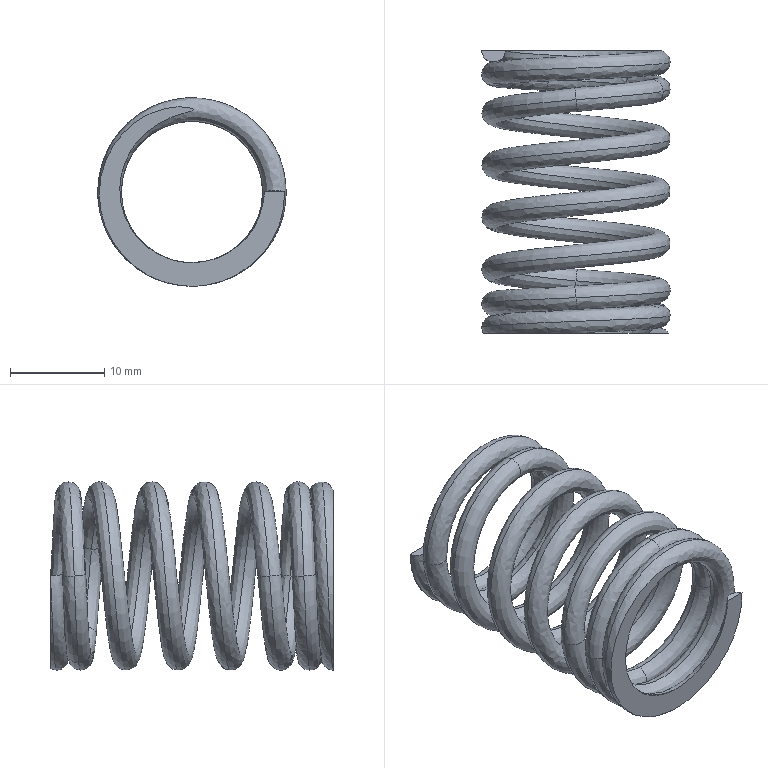Part | STEP file | Compress Spring1_5 | 1 solid | 26 faces | volume 1934 mm3 | spline 22 | plane 4